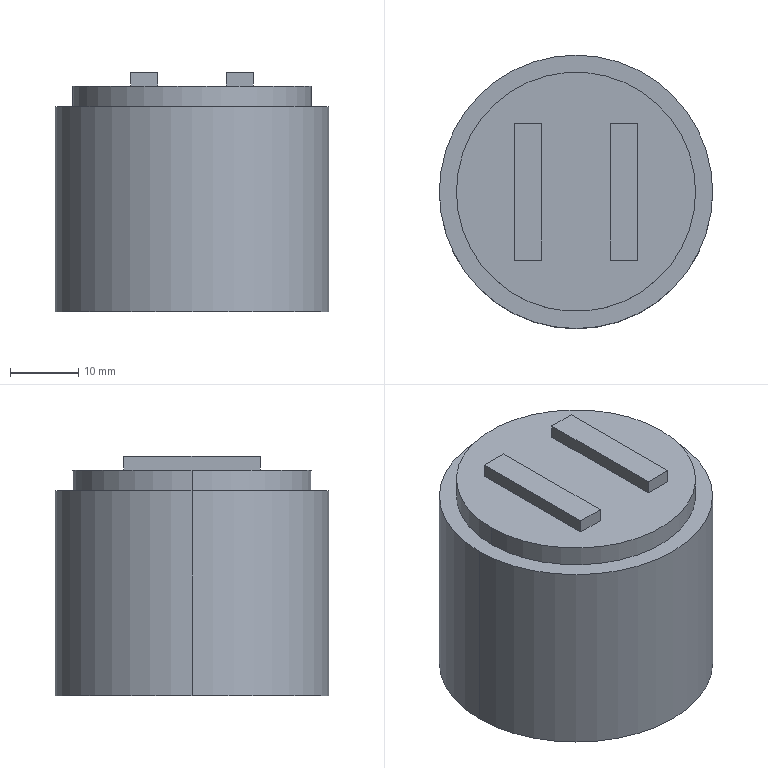Part | SolidWorks | features MBimport 1 | 1 solid | 17 faces | box 40 x 40 x 35 mm | volume 40905 mm3 | plane 13 | cylinder 4 | commonest cylinder face diameters 35 x2 40 x2
STEP:
#1=CARTESIAN_POINT('',(-20.,0.,0.));
#2=VERTEX_POINT('',#1);
#3=CARTESIAN_POINT('',(20.,0.,0.));
#4=VERTEX_POINT('',#3);
#5=CARTESIAN_POINT('',(0.,0.,0.));
#6=DIRECTION('',(0.,0.,1.));
#7=DIRECTION('',(-1.,0.,0.));
#8=AXIS2_PLACEMENT_3D('',#5,#6,#7);
#9=CIRCLE('',#8,20.);
#10=EDGE_CURVE('',#2,#4,#9,.T.);
#11=ORIENTED_EDGE('',*,*,#10,.F.);
#12=CARTESIAN_POINT('',(0.,0.,0.));
#13=DIRECTION('',(0.,0.,1.));
#14=DIRECTION('',(1.,0.,0.));
#15=AXIS2_PLACEMENT_3D('',#12,#13,#14);
#16=CIRCLE('',#15,20.);
#17=EDGE_CURVE('',#4,#2,#16,.T.);
#18=ORIENTED_EDGE('',*,*,#17,.F.);
#19=EDGE_LOOP('',(#11,#18));
#20=FACE_OUTER_BOUND('',#19,.T.);
#21=CARTESIAN_POINT('',(0.,0.,0.));
#22=DIRECTION('',(0.,0.,1.));
#23=DIRECTION('',(1.,0.,0.));
#24=AXIS2_PLACEMENT_3D('',#21,#22,#23);
#25=PLANE('',#24);
#26=ADVANCED_FACE('',(#20),#25,.F.);
#27=CARTESIAN_POINT('',(20.,0.,30.));
#28=VERTEX_POINT('',#27);
#29=CARTESIAN_POINT('',(20.,0.,0.));
#30=DIRECTION('',(0.,0.,1.));
#31=VECTOR('',#30,1000.);
#32=LINE('',#29,#31);
#33=EDGE_CURVE('',#4,#28,#32,.T.);
#34=ORIENTED_EDGE('',*,*,#33,.T.);
#35=CARTESIAN_POINT('',(-20.,0.,30.));
#36=VERTEX_POINT('',#35);
#37=CARTESIAN_POINT('',(0.,0.,30.));
#38=DIRECTION('',(0.,0.,1.));
#39=DIRECTION('',(-1.,0.,0.));
#40=AXIS2_PLACEMENT_3D('',#37,#38,#39);
#41=CIRCLE('',#40,20.);
#42=EDGE_CURVE('',#36,#28,#41,.T.);
#43=ORIENTED_EDGE('',*,*,#42,.F.);
#44=CARTESIAN_POINT('',(-20.,0.,0.));
#45=DIRECTION('',(0.,0.,1.));
#46=VECTOR('',#45,1000.);
#47=LINE('',#44,#46);
#48=EDGE_CURVE('',#2,#36,#47,.T.);
#49=ORIENTED_EDGE('',*,*,#48,.F.);
#50=ORIENTED_EDGE('',*,*,#10,.T.);
#51=EDGE_LOOP('',(#34,#43,#49,#50));
#52=FACE_OUTER_BOUND('',#51,.T.);
#53=CARTESIAN_POINT('',(0.,0.,0.));
#54=DIRECTION('',(0.,0.,-1.));
#55=DIRECTION('',(1.,0.,0.));
#56=AXIS2_PLACEMENT_3D('',#53,#54,#55);
#57=CYLINDRICAL_SURFACE('',#56,20.);
#58=ADVANCED_FACE('',(#52),#57,.T.);
#59=ORIENTED_EDGE('',*,*,#48,.T.);
#60=CARTESIAN_POINT('',(0.,0.,30.));
#61=DIRECTION('',(0.,0.,1.));
#62=DIRECTION('',(1.,0.,0.));
#63=AXIS2_PLACEMENT_3D('',#60,#61,#62);
#64=CIRCLE('',#63,20.);
#65=EDGE_CURVE('',#28,#36,#64,.T.);
#66=ORIENTED_EDGE('',*,*,#65,.F.);
#67=ORIENTED_EDGE('',*,*,#33,.F.);
#68=ORIENTED_EDGE('',*,*,#17,.T.);
#69=EDGE_LOOP('',(#59,#66,#67,#68));
#70=FACE_OUTER_BOUND('',#69,.T.);
#71=CARTESIAN_POINT('',(0.,0.,0.));
#72=DIRECTION('',(0.,0.,-1.));
#73=DIRECTION('',(1.,0.,0.));
#74=AXIS2_PLACEMENT_3D('',#71,#72,#73);
#75=CYLINDRICAL_SURFACE('',#74,20.);
#76=ADVANCED_FACE('',(#70),#75,.T.);
#77=CARTESIAN_POINT('',(-17.5,0.,30.));
#78=VERTEX_POINT('',#77);
#79=CARTESIAN_POINT('',(17.5,0.,30.));
#80=VERTEX_POINT('',#79);
#81=CARTESIAN_POINT('',(0.,0.,30.));
#82=DIRECTION('',(0.,0.,1.));
#83=DIRECTION('',(-1.,0.,0.));
#84=AXIS2_PLACEMENT_3D('',#81,#82,#83);
#85=CIRCLE('',#84,17.5);
#86=EDGE_CURVE('',#78,#80,#85,.T.);
#87=ORIENTED_EDGE('',*,*,#86,.F.);
#88=CARTESIAN_POINT('',(0.,0.,30.));
#89=DIRECTION('',(0.,0.,1.));
#90=DIRECTION('',(1.,0.,0.));
#91=AXIS2_PLACEMENT_3D('',#88,#89,#90);
#92=CIRCLE('',#91,17.5);
#93=EDGE_CURVE('',#80,#78,#92,.T.);
#94=ORIENTED_EDGE('',*,*,#93,.F.);
#95=EDGE_LOOP('',(#87,#94));
#96=FACE_BOUND('',#95,.T.);
#97=ORIENTED_EDGE('',*,*,#42,.T.);
#98=ORIENTED_EDGE('',*,*,#65,.T.);
#99=EDGE_LOOP('',(#97,#98));
#100=FACE_OUTER_BOUND('',#99,.T.);
#101=CARTESIAN_POINT('',(0.,0.,30.));
#102=DIRECTION('',(0.,0.,1.));
#103=DIRECTION('',(1.,0.,0.));
#104=AXIS2_PLACEMENT_3D('',#101,#102,#103);
#105=PLANE('',#104);
#106=ADVANCED_FACE('',(#96,#100),#105,.T.);
#107=CARTESIAN_POINT('',(17.5,0.,33.));
#108=VERTEX_POINT('',#107);
#109=CARTESIAN_POINT('',(17.5,0.,30.));
#110=DIRECTION('',(0.,0.,1.));
#111=VECTOR('',#110,1000.);
#112=LINE('',#109,#111);
#113=EDGE_CURVE('',#80,#108,#112,.T.);
#114=ORIENTED_EDGE('',*,*,#113,.T.);
#115=CARTESIAN_POINT('',(-17.5,0.,33.));
#116=VERTEX_POINT('',#115);
#117=CARTESIAN_POINT('',(0.,0.,33.));
#118=DIRECTION('',(0.,0.,1.));
#119=DIRECTION('',(-1.,0.,0.));
#120=AXIS2_PLACEMENT_3D('',#117,#118,#119);
#121=CIRCLE('',#120,17.5);
#122=EDGE_CURVE('',#116,#108,#121,.T.);
#123=ORIENTED_EDGE('',*,*,#122,.F.);
#124=CARTESIAN_POINT('',(-17.5,0.,30.));
#125=DIRECTION('',(0.,0.,1.));
#126=VECTOR('',#125,1000.);
#127=LINE('',#124,#126);
#128=EDGE_CURVE('',#78,#116,#127,.T.);
#129=ORIENTED_EDGE('',*,*,#128,.F.);
#130=ORIENTED_EDGE('',*,*,#86,.T.);
#131=EDGE_LOOP('',(#114,#123,#129,#130));
#132=FACE_OUTER_BOUND('',#131,.T.);
#133=CARTESIAN_POINT('',(0.,0.,30.));
#134=DIRECTION('',(0.,0.,-1.));
#135=DIRECTION('',(1.,0.,0.));
#136=AXIS2_PLACEMENT_3D('',#133,#134,#135);
#137=CYLINDRICAL_SURFACE('',#136,17.5);
#138=ADVANCED_FACE('',(#132),#137,.T.);
#139=ORIENTED_EDGE('',*,*,#128,.T.);
#140=CARTESIAN_POINT('',(0.,0.,33.));
#141=DIRECTION('',(0.,0.,1.));
#142=DIRECTION('',(1.,0.,0.));
#143=AXIS2_PLACEMENT_3D('',#140,#141,#142);
#144=CIRCLE('',#143,17.5);
#145=EDGE_CURVE('',#108,#116,#144,.T.);
#146=ORIENTED_EDGE('',*,*,#145,.F.);
#147=ORIENTED_EDGE('',*,*,#113,.F.);
#148=ORIENTED_EDGE('',*,*,#93,.T.);
#149=EDGE_LOOP('',(#139,#146,#147,#148));
#150=FACE_OUTER_BOUND('',#149,.T.);
#151=CARTESIAN_POINT('',(0.,0.,30.));
#152=DIRECTION('',(0.,0.,-1.));
#153=DIRECTION('',(1.,0.,0.));
#154=AXIS2_PLACEMENT_3D('',#151,#152,#153);
#155=CYLINDRICAL_SURFACE('',#154,17.5);
#156=ADVANCED_FACE('',(#150),#155,.T.);
#157=CARTESIAN_POINT('',(-5.,10.,33.));
#158=VERTEX_POINT('',#157);
#159=CARTESIAN_POINT('',(-5.,-10.,33.));
#160=VERTEX_POINT('',#159);
#161=CARTESIAN_POINT('',(-5.,10.,33.));
#162=DIRECTION('',(0.,-1.,0.));
#163=VECTOR('',#162,1000.);
#164=LINE('',#161,#163);
#165=EDGE_CURVE('',#158,#160,#164,.T.);
#166=ORIENTED_EDGE('',*,*,#165,.T.);
#167=CARTESIAN_POINT('',(-9.,-10.,33.));
#168=VERTEX_POINT('',#167);
#169=CARTESIAN_POINT('',(-5.,-10.,33.));
#170=DIRECTION('',(-1.,0.,0.));
#171=VECTOR('',#170,1000.);
#172=LINE('',#169,#171);
#173=EDGE_CURVE('',#160,#168,#172,.T.);
#174=ORIENTED_EDGE('',*,*,#173,.T.);
#175=CARTESIAN_POINT('',(-9.,10.,33.));
#176=VERTEX_POINT('',#175);
#177=CARTESIAN_POINT('',(-9.,-10.,33.));
#178=DIRECTION('',(0.,1.,0.));
#179=VECTOR('',#178,1000.);
#180=LINE('',#177,#179);
#181=EDGE_CURVE('',#168,#176,#180,.T.);
#182=ORIENTED_EDGE('',*,*,#181,.T.);
#183=CARTESIAN_POINT('',(-9.,10.,33.));
#184=DIRECTION('',(1.,0.,0.));
#185=VECTOR('',#184,1000.);
#186=LINE('',#183,#185);
#187=EDGE_CURVE('',#176,#158,#186,.T.);
#188=ORIENTED_EDGE('',*,*,#187,.T.);
#189=EDGE_LOOP('',(#166,#174,#182,#188));
#190=FACE_BOUND('',#189,.T.);
#191=CARTESIAN_POINT('',(9.,-10.,33.));
#192=VERTEX_POINT('',#191);
#193=CARTESIAN_POINT('',(9.,10.,33.));
#194=VERTEX_POINT('',#193);
#195=CARTESIAN_POINT('',(9.,-10.,33.));
#196=DIRECTION('',(0.,1.,0.));
#197=VECTOR('',#196,1000.);
#198=LINE('',#195,#197);
#199=EDGE_CURVE('',#192,#194,#198,.T.);
#200=ORIENTED_EDGE('',*,*,#199,.F.);
#201=CARTESIAN_POINT('',(5.,-10.,33.));
#202=VERTEX_POINT('',#201);
#203=CARTESIAN_POINT('',(5.,-10.,33.));
#204=DIRECTION('',(1.,0.,0.));
#205=VECTOR('',#204,1000.);
#206=LINE('',#203,#205);
#207=EDGE_CURVE('',#202,#192,#206,.T.);
#208=ORIENTED_EDGE('',*,*,#207,.F.);
#209=CARTESIAN_POINT('',(5.,10.,33.));
#210=VERTEX_POINT('',#209);
#211=CARTESIAN_POINT('',(5.,10.,33.));
#212=DIRECTION('',(0.,-1.,0.));
#213=VECTOR('',#212,1000.);
#214=LINE('',#211,#213);
#215=EDGE_CURVE('',#210,#202,#214,.T.);
#216=ORIENTED_EDGE('',*,*,#215,.F.);
#217=CARTESIAN_POINT('',(9.,10.,33.));
#218=DIRECTION('',(-1.,0.,0.));
#219=VECTOR('',#218,1000.);
#220=LINE('',#217,#219);
#221=EDGE_CURVE('',#194,#210,#220,.T.);
#222=ORIENTED_EDGE('',*,*,#221,.F.);
#223=EDGE_LOOP('',(#200,#208,#216,#222));
#224=FACE_BOUND('',#223,.T.);
#225=ORIENTED_EDGE('',*,*,#122,.T.);
#226=ORIENTED_EDGE('',*,*,#145,.T.);
#227=EDGE_LOOP('',(#225,#226));
#228=FACE_OUTER_BOUND('',#227,.T.);
#229=CARTESIAN_POINT('',(0.,0.,33.));
#230=DIRECTION('',(0.,0.,1.));
#231=DIRECTION('',(1.,0.,0.));
#232=AXIS2_PLACEMENT_3D('',#229,#230,#231);
#233=PLANE('',#232);
#234=ADVANCED_FACE('',(#190,#224,#228),#233,.T.);
#235=CARTESIAN_POINT('',(-5.,10.,35.));
#236=VERTEX_POINT('',#235);
#237=CARTESIAN_POINT('',(-5.,-10.,35.));
#238=VERTEX_POINT('',#237);
#239=CARTESIAN_POINT('',(-5.,10.,35.));
#240=DIRECTION('',(0.,-1.,0.));
#241=VECTOR('',#240,1000.);
#242=LINE('',#239,#241);
#243=EDGE_CURVE('',#236,#238,#242,.T.);
#244=ORIENTED_EDGE('',*,*,#243,.T.);
#245=CARTESIAN_POINT('',(-5.,-10.,33.));
#246=DIRECTION('',(0.,0.,1.));
#247=VECTOR('',#246,1000.);
#248=LINE('',#245,#247);
#249=EDGE_CURVE('',#160,#238,#248,.T.);
#250=ORIENTED_EDGE('',*,*,#249,.F.);
#251=ORIENTED_EDGE('',*,*,#165,.F.);
#252=CARTESIAN_POINT('',(-5.,10.,33.));
#253=DIRECTION('',(0.,0.,1.));
#254=VECTOR('',#253,1000.);
#255=LINE('',#252,#254);
#256=EDGE_CURVE('',#158,#236,#255,.T.);
#257=ORIENTED_EDGE('',*,*,#256,.T.);
#258=EDGE_LOOP('',(#244,#250,#251,#257));
#259=FACE_OUTER_BOUND('',#258,.T.);
#260=CARTESIAN_POINT('',(-5.,10.,33.));
#261=DIRECTION('',(-1.,0.,0.));
#262=DIRECTION('',(0.,-1.,0.));
#263=AXIS2_PLACEMENT_3D('',#260,#261,#262);
#264=PLANE('',#263);
#265=ADVANCED_FACE('',(#259),#264,.F.);
#266=CARTESIAN_POINT('',(-9.,-10.,35.));
#267=VERTEX_POINT('',#266);
#268=CARTESIAN_POINT('',(-5.,-10.,35.));
#269=DIRECTION('',(-1.,0.,0.));
#270=VECTOR('',#269,1000.);
#271=LINE('',#268,#270);
#272=EDGE_CURVE('',#238,#267,#271,.T.);
#273=ORIENTED_EDGE('',*,*,#272,.T.);
#274=CARTESIAN_POINT('',(-9.,-10.,33.));
#275=DIRECTION('',(0.,0.,1.));
#276=VECTOR('',#275,1000.);
#277=LINE('',#274,#276);
#278=EDGE_CURVE('',#168,#267,#277,.T.);
#279=ORIENTED_EDGE('',*,*,#278,.F.);
#280=ORIENTED_EDGE('',*,*,#173,.F.);
#281=ORIENTED_EDGE('',*,*,#249,.T.);
#282=EDGE_LOOP('',(#273,#279,#280,#281));
#283=FACE_OUTER_BOUND('',#282,.T.);
#284=CARTESIAN_POINT('',(-5.,-10.,33.));
#285=DIRECTION('',(0.,1.,0.));
#286=DIRECTION('',(-1.,0.,0.));
#287=AXIS2_PLACEMENT_3D('',#284,#285,#286);
#288=PLANE('',#287);
#289=ADVANCED_FACE('',(#283),#288,.F.);
#290=ORIENTED_EDGE('',*,*,#181,.F.);
#291=ORIENTED_EDGE('',*,*,#278,.T.);
#292=CARTESIAN_POINT('',(-9.,10.,35.));
#293=VERTEX_POINT('',#292);
#294=CARTESIAN_POINT('',(-9.,-10.,35.));
#295=DIRECTION('',(0.,1.,0.));
#296=VECTOR('',#295,1000.);
#297=LINE('',#294,#296);
#298=EDGE_CURVE('',#267,#293,#297,.T.);
#299=ORIENTED_EDGE('',*,*,#298,.T.);
#300=CARTESIAN_POINT('',(-9.,10.,33.));
#301=DIRECTION('',(0.,0.,1.));
#302=VECTOR('',#301,1000.);
#303=LINE('',#300,#302);
#304=EDGE_CURVE('',#176,#293,#303,.T.);
#305=ORIENTED_EDGE('',*,*,#304,.F.);
#306=EDGE_LOOP('',(#290,#291,#299,#305));
#307=FACE_OUTER_BOUND('',#306,.T.);
#308=CARTESIAN_POINT('',(-9.,-10.,33.));
#309=DIRECTION('',(1.,0.,0.));
#310=DIRECTION('',(0.,1.,0.));
#311=AXIS2_PLACEMENT_3D('',#308,#309,#310);
#312=PLANE('',#311);
#313=ADVANCED_FACE('',(#307),#312,.F.);
#314=CARTESIAN_POINT('',(-9.,10.,35.));
#315=DIRECTION('',(1.,0.,0.));
#316=VECTOR('',#315,1000.);
#317=LINE('',#314,#316);
#318=EDGE_CURVE('',#293,#236,#317,.T.);
#319=ORIENTED_EDGE('',*,*,#318,.T.);
#320=ORIENTED_EDGE('',*,*,#256,.F.);
#321=ORIENTED_EDGE('',*,*,#187,.F.);
#322=ORIENTED_EDGE('',*,*,#304,.T.);
#323=EDGE_LOOP('',(#319,#320,#321,#322));
#324=FACE_OUTER_BOUND('',#323,.T.);
#325=CARTESIAN_POINT('',(-9.,10.,33.));
#326=DIRECTION('',(0.,-1.,0.));
#327=DIRECTION('',(1.,0.,0.));
#328=AXIS2_PLACEMENT_3D('',#325,#326,#327);
#329=PLANE('',#328);
#330=ADVANCED_FACE('',(#324),#329,.F.);
#331=CARTESIAN_POINT('',(9.,10.,35.));
#332=VERTEX_POINT('',#331);
#333=CARTESIAN_POINT('',(9.,10.,33.));
#334=DIRECTION('',(0.,0.,1.));
#335=VECTOR('',#334,1000.);
#336=LINE('',#333,#335);
#337=EDGE_CURVE('',#194,#332,#336,.T.);
#338=ORIENTED_EDGE('',*,*,#337,.T.);
#339=CARTESIAN_POINT('',(9.,-10.,35.));
#340=VERTEX_POINT('',#339);
#341=CARTESIAN_POINT('',(9.,-10.,35.));
#342=DIRECTION('',(0.,1.,0.));
#343=VECTOR('',#342,1000.);
#344=LINE('',#341,#343);
#345=EDGE_CURVE('',#340,#332,#344,.T.);
#346=ORIENTED_EDGE('',*,*,#345,.F.);
#347=CARTESIAN_POINT('',(9.,-10.,33.));
#348=DIRECTION('',(0.,0.,1.));
#349=VECTOR('',#348,1000.);
#350=LINE('',#347,#349);
#351=EDGE_CURVE('',#192,#340,#350,.T.);
#352=ORIENTED_EDGE('',*,*,#351,.F.);
#353=ORIENTED_EDGE('',*,*,#199,.T.);
#354=EDGE_LOOP('',(#338,#346,#352,#353));
#355=FACE_OUTER_BOUND('',#354,.T.);
#356=CARTESIAN_POINT('',(9.,-10.,33.));
#357=DIRECTION('',(1.,0.,0.));
#358=DIRECTION('',(0.,1.,0.));
#359=AXIS2_PLACEMENT_3D('',#356,#357,#358);
#360=PLANE('',#359);
#361=ADVANCED_FACE('',(#355),#360,.T.);
#362=ORIENTED_EDGE('',*,*,#351,.T.);
#363=CARTESIAN_POINT('',(5.,-10.,35.));
#364=VERTEX_POINT('',#363);
#365=CARTESIAN_POINT('',(5.,-10.,35.));
#366=DIRECTION('',(1.,0.,0.));
#367=VECTOR('',#366,1000.);
#368=LINE('',#365,#367);
#369=EDGE_CURVE('',#364,#340,#368,.T.);
#370=ORIENTED_EDGE('',*,*,#369,.F.);
#371=CARTESIAN_POINT('',(5.,-10.,33.));
#372=DIRECTION('',(0.,0.,1.));
#373=VECTOR('',#372,1000.);
#374=LINE('',#371,#373);
#375=EDGE_CURVE('',#202,#364,#374,.T.);
#376=ORIENTED_EDGE('',*,*,#375,.F.);
#377=ORIENTED_EDGE('',*,*,#207,.T.);
#378=EDGE_LOOP('',(#362,#370,#376,#377));
#379=FACE_OUTER_BOUND('',#378,.T.);
#380=CARTESIAN_POINT('',(5.,-10.,33.));
#381=DIRECTION('',(0.,-1.,0.));
#382=DIRECTION('',(1.,0.,0.));
#383=AXIS2_PLACEMENT_3D('',#380,#381,#382);
#384=PLANE('',#383);
#385=ADVANCED_FACE('',(#379),#384,.T.);
#386=ORIENTED_EDGE('',*,*,#375,.T.);
#387=CARTESIAN_POINT('',(5.,10.,35.));
#388=VERTEX_POINT('',#387);
#389=CARTESIAN_POINT('',(5.,10.,35.));
#390=DIRECTION('',(0.,-1.,0.));
#391=VECTOR('',#390,1000.);
#392=LINE('',#389,#391);
#393=EDGE_CURVE('',#388,#364,#392,.T.);
#394=ORIENTED_EDGE('',*,*,#393,.F.);
#395=CARTESIAN_POINT('',(5.,10.,33.));
#396=DIRECTION('',(0.,0.,1.));
#397=VECTOR('',#396,1000.);
#398=LINE('',#395,#397);
#399=EDGE_CURVE('',#210,#388,#398,.T.);
#400=ORIENTED_EDGE('',*,*,#399,.F.);
#401=ORIENTED_EDGE('',*,*,#215,.T.);
#402=EDGE_LOOP('',(#386,#394,#400,#401));
#403=FACE_OUTER_BOUND('',#402,.T.);
#404=CARTESIAN_POINT('',(5.,10.,33.));
#405=DIRECTION('',(-1.,0.,0.));
#406=DIRECTION('',(0.,-1.,0.));
#407=AXIS2_PLACEMENT_3D('',#404,#405,#406);
#408=PLANE('',#407);
#409=ADVANCED_FACE('',(#403),#408,.T.);
#410=ORIENTED_EDGE('',*,*,#399,.T.);
#411=CARTESIAN_POINT('',(9.,10.,35.));
#412=DIRECTION('',(-1.,0.,0.));
#413=VECTOR('',#412,1000.);
#414=LINE('',#411,#413);
#415=EDGE_CURVE('',#332,#388,#414,.T.);
#416=ORIENTED_EDGE('',*,*,#415,.F.);
#417=ORIENTED_EDGE('',*,*,#337,.F.);
#418=ORIENTED_EDGE('',*,*,#221,.T.);
#419=EDGE_LOOP('',(#410,#416,#417,#418));
#420=FACE_OUTER_BOUND('',#419,.T.);
#421=CARTESIAN_POINT('',(9.,10.,33.));
#422=DIRECTION('',(0.,1.,0.));
#423=DIRECTION('',(-1.,0.,0.));
#424=AXIS2_PLACEMENT_3D('',#421,#422,#423);
#425=PLANE('',#424);
#426=ADVANCED_FACE('',(#420),#425,.T.);
#427=ORIENTED_EDGE('',*,*,#298,.F.);
#428=ORIENTED_EDGE('',*,*,#272,.F.);
#429=ORIENTED_EDGE('',*,*,#243,.F.);
#430=ORIENTED_EDGE('',*,*,#318,.F.);
#431=EDGE_LOOP('',(#427,#428,#429,#430));
#432=FACE_OUTER_BOUND('',#431,.T.);
#433=CARTESIAN_POINT('',(0.,0.,35.));
#434=DIRECTION('',(0.,0.,-1.));
#435=DIRECTION('',(-1.,0.,0.));
#436=AXIS2_PLACEMENT_3D('',#433,#434,#435);
#437=PLANE('',#436);
#438=ADVANCED_FACE('',(#432),#437,.F.);
#439=ORIENTED_EDGE('',*,*,#393,.T.);
#440=ORIENTED_EDGE('',*,*,#369,.T.);
#441=ORIENTED_EDGE('',*,*,#345,.T.);
#442=ORIENTED_EDGE('',*,*,#415,.T.);
#443=EDGE_LOOP('',(#439,#440,#441,#442));
#444=FACE_OUTER_BOUND('',#443,.T.);
#445=CARTESIAN_POINT('',(0.,0.,35.));
#446=DIRECTION('',(0.,0.,1.));
#447=DIRECTION('',(1.,0.,0.));
#448=AXIS2_PLACEMENT_3D('',#445,#446,#447);
#449=PLANE('',#448);
#450=ADVANCED_FACE('',(#444),#449,.T.);
#451=CLOSED_SHELL('',(#26,#58,#76,#106,#138,#156,#234,#265,#289,#313,#330,#361,#385,#409,#426,#438,#450));
#452=MANIFOLD_SOLID_BREP('',#451);
#453=CARTESIAN_POINT('',(0.,0.,0.));
#454=DIRECTION('',(0.,0.,1.));
#455=DIRECTION('',(1.,0.,0.));
#456=AXIS2_PLACEMENT_3D('',#453,#454,#455);
#457=(LENGTH_UNIT()NAMED_UNIT(*)SI_UNIT(.MILLI.,.METRE.));
#458=UNCERTAINTY_MEASURE_WITH_UNIT(LENGTH_MEASURE(0.00001),#457,'','');
#459=(NAMED_UNIT(*)PLANE_ANGLE_UNIT()SI_UNIT($,.RADIAN.));
#460=(NAMED_UNIT(*)SI_UNIT($,.STERADIAN.)SOLID_ANGLE_UNIT());
#461=(GEOMETRIC_REPRESENTATION_CONTEXT(3)GLOBAL_UNCERTAINTY_ASSIGNED_CONTEXT((#458))GLOBAL_UNIT_ASSIGNED_CONTEXT((#457,#459,#460))REPRESENTATION_CONTEXT('',''));
#462=ADVANCED_BREP_SHAPE_REPRESENTATION('',(#452,#456),#461);